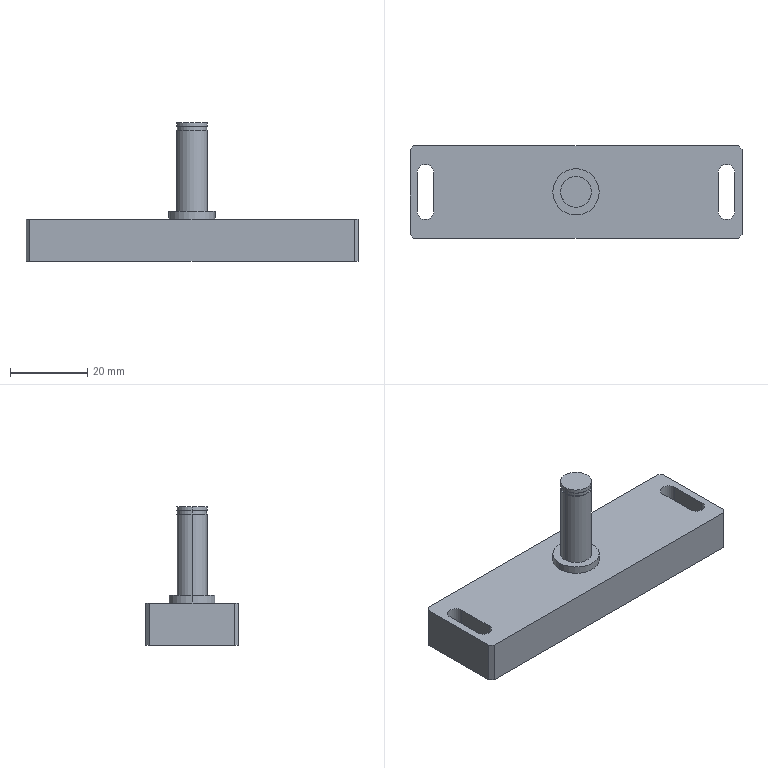Part | SolidWorks | features ICE 7, Chamfer 1, Extrusion 1, RevCut 1 | 1 solid | 30 faces | box 86 x 24 x 36 mm | volume 22794 mm3 | plane 18 | cylinder 12 | commonest cylinder face diameters 4.3 x4 8 x4 7.6 x2 12 x2
STEP:
#1=CARTESIAN_POINT('',(-4.,0.,28.5));
#2=VERTEX_POINT('',#1);
#3=CARTESIAN_POINT('',(4.,0.,28.5));
#4=VERTEX_POINT('',#3);
#5=CARTESIAN_POINT('',(0.,0.,28.5));
#6=DIRECTION('',(0.,0.,-1.));
#7=DIRECTION('',(-1.,0.,0.));
#8=AXIS2_PLACEMENT_3D('',#5,#6,#7);
#9=CIRCLE('',#8,4.);
#10=EDGE_CURVE('',#2,#4,#9,.T.);
#11=ORIENTED_EDGE('',*,*,#10,.T.);
#12=CARTESIAN_POINT('',(4.,0.,7.5));
#13=VERTEX_POINT('',#12);
#14=CARTESIAN_POINT('',(4.,0.,9.));
#15=DIRECTION('',(0.,0.,-1.));
#16=VECTOR('',#15,1000.);
#17=LINE('',#14,#16);
#18=EDGE_CURVE('',#4,#13,#17,.T.);
#19=ORIENTED_EDGE('',*,*,#18,.T.);
#20=CARTESIAN_POINT('',(-4.,0.,7.5));
#21=VERTEX_POINT('',#20);
#22=CARTESIAN_POINT('',(0.,0.,7.5));
#23=DIRECTION('',(0.,0.,1.));
#24=DIRECTION('',(1.,0.,0.));
#25=AXIS2_PLACEMENT_3D('',#22,#23,#24);
#26=CIRCLE('',#25,4.);
#27=EDGE_CURVE('',#13,#21,#26,.T.);
#28=ORIENTED_EDGE('',*,*,#27,.T.);
#29=CARTESIAN_POINT('',(-4.,0.,9.));
#30=DIRECTION('',(0.,0.,-1.));
#31=VECTOR('',#30,1000.);
#32=LINE('',#29,#31);
#33=EDGE_CURVE('',#2,#21,#32,.T.);
#34=ORIENTED_EDGE('',*,*,#33,.F.);
#35=EDGE_LOOP('',(#11,#19,#28,#34));
#36=FACE_OUTER_BOUND('',#35,.T.);
#37=CARTESIAN_POINT('',(0.,0.,9.));
#38=DIRECTION('',(0.,0.,-1.));
#39=DIRECTION('',(-1.,0.,0.));
#40=AXIS2_PLACEMENT_3D('',#37,#38,#39);
#41=CYLINDRICAL_SURFACE('',#40,4.);
#42=ADVANCED_FACE('',(#36),#41,.T.);
#43=CARTESIAN_POINT('',(-3.8,0.,29.5));
#44=VERTEX_POINT('',#43);
#45=CARTESIAN_POINT('',(3.8,0.,29.5));
#46=VERTEX_POINT('',#45);
#47=CARTESIAN_POINT('',(0.,0.,29.5));
#48=DIRECTION('',(0.,0.,-1.));
#49=DIRECTION('',(-1.,0.,0.));
#50=AXIS2_PLACEMENT_3D('',#47,#48,#49);
#51=CIRCLE('',#50,3.8);
#52=EDGE_CURVE('',#44,#46,#51,.T.);
#53=ORIENTED_EDGE('',*,*,#52,.T.);
#54=CARTESIAN_POINT('',(3.8,0.,28.5));
#55=VERTEX_POINT('',#54);
#56=CARTESIAN_POINT('',(3.8,0.,0.));
#57=DIRECTION('',(0.,0.,-1.));
#58=VECTOR('',#57,1000.);
#59=LINE('',#56,#58);
#60=EDGE_CURVE('',#46,#55,#59,.T.);
#61=ORIENTED_EDGE('',*,*,#60,.T.);
#62=CARTESIAN_POINT('',(-3.8,0.,28.5));
#63=VERTEX_POINT('',#62);
#64=CARTESIAN_POINT('',(0.,0.,28.5));
#65=DIRECTION('',(0.,0.,-1.));
#66=DIRECTION('',(-1.,0.,0.));
#67=AXIS2_PLACEMENT_3D('',#64,#65,#66);
#68=CIRCLE('',#67,3.8);
#69=EDGE_CURVE('',#63,#55,#68,.T.);
#70=ORIENTED_EDGE('',*,*,#69,.F.);
#71=CARTESIAN_POINT('',(-3.8,0.,0.));
#72=DIRECTION('',(0.,0.,-1.));
#73=VECTOR('',#72,1000.);
#74=LINE('',#71,#73);
#75=EDGE_CURVE('',#44,#63,#74,.T.);
#76=ORIENTED_EDGE('',*,*,#75,.F.);
#77=EDGE_LOOP('',(#53,#61,#70,#76));
#78=FACE_OUTER_BOUND('',#77,.T.);
#79=CARTESIAN_POINT('',(0.,0.,0.));
#80=DIRECTION('',(0.,0.,-1.));
#81=DIRECTION('',(-1.,0.,0.));
#82=AXIS2_PLACEMENT_3D('',#79,#80,#81);
#83=CYLINDRICAL_SURFACE('',#82,3.8);
#84=ADVANCED_FACE('',(#78),#83,.T.);
#85=CARTESIAN_POINT('',(4.,0.,30.5));
#86=VERTEX_POINT('',#85);
#87=CARTESIAN_POINT('',(-4.,0.,30.5));
#88=VERTEX_POINT('',#87);
#89=CARTESIAN_POINT('',(0.,0.,30.5));
#90=DIRECTION('',(0.,0.,1.));
#91=DIRECTION('',(1.,0.,0.));
#92=AXIS2_PLACEMENT_3D('',#89,#90,#91);
#93=CIRCLE('',#92,4.);
#94=EDGE_CURVE('',#86,#88,#93,.T.);
#95=ORIENTED_EDGE('',*,*,#94,.F.);
#96=CARTESIAN_POINT('',(4.,0.,29.5));
#97=VERTEX_POINT('',#96);
#98=CARTESIAN_POINT('',(4.,0.,9.));
#99=DIRECTION('',(0.,0.,-1.));
#100=VECTOR('',#99,1000.);
#101=LINE('',#98,#100);
#102=EDGE_CURVE('',#86,#97,#101,.T.);
#103=ORIENTED_EDGE('',*,*,#102,.T.);
#104=CARTESIAN_POINT('',(-4.,0.,29.5));
#105=VERTEX_POINT('',#104);
#106=CARTESIAN_POINT('',(0.,0.,29.5));
#107=DIRECTION('',(0.,0.,-1.));
#108=DIRECTION('',(-1.,0.,0.));
#109=AXIS2_PLACEMENT_3D('',#106,#107,#108);
#110=CIRCLE('',#109,4.);
#111=EDGE_CURVE('',#105,#97,#110,.T.);
#112=ORIENTED_EDGE('',*,*,#111,.F.);
#113=CARTESIAN_POINT('',(-4.,0.,9.));
#114=DIRECTION('',(0.,0.,-1.));
#115=VECTOR('',#114,1000.);
#116=LINE('',#113,#115);
#117=EDGE_CURVE('',#88,#105,#116,.T.);
#118=ORIENTED_EDGE('',*,*,#117,.F.);
#119=EDGE_LOOP('',(#95,#103,#112,#118));
#120=FACE_OUTER_BOUND('',#119,.T.);
#121=CARTESIAN_POINT('',(0.,0.,9.));
#122=DIRECTION('',(0.,0.,-1.));
#123=DIRECTION('',(-1.,0.,0.));
#124=AXIS2_PLACEMENT_3D('',#121,#122,#123);
#125=CYLINDRICAL_SURFACE('',#124,4.);
#126=ADVANCED_FACE('',(#120),#125,.T.);
#127=CARTESIAN_POINT('',(6.,0.,7.5));
#128=VERTEX_POINT('',#127);
#129=CARTESIAN_POINT('',(-6.,0.,7.5));
#130=VERTEX_POINT('',#129);
#131=CARTESIAN_POINT('',(0.,0.,7.5));
#132=DIRECTION('',(0.,0.,1.));
#133=DIRECTION('',(1.,0.,0.));
#134=AXIS2_PLACEMENT_3D('',#131,#132,#133);
#135=CIRCLE('',#134,6.);
#136=EDGE_CURVE('',#128,#130,#135,.T.);
#137=ORIENTED_EDGE('',*,*,#136,.F.);
#138=CARTESIAN_POINT('',(6.,0.,5.5));
#139=VERTEX_POINT('',#138);
#140=CARTESIAN_POINT('',(6.,0.,7.5));
#141=DIRECTION('',(0.,0.,-1.));
#142=VECTOR('',#141,1000.);
#143=LINE('',#140,#142);
#144=EDGE_CURVE('',#128,#139,#143,.T.);
#145=ORIENTED_EDGE('',*,*,#144,.T.);
#146=CARTESIAN_POINT('',(-6.,0.,5.5));
#147=VERTEX_POINT('',#146);
#148=CARTESIAN_POINT('',(0.,0.,5.5));
#149=DIRECTION('',(0.,0.,1.));
#150=DIRECTION('',(1.,0.,0.));
#151=AXIS2_PLACEMENT_3D('',#148,#149,#150);
#152=CIRCLE('',#151,6.);
#153=EDGE_CURVE('',#139,#147,#152,.T.);
#154=ORIENTED_EDGE('',*,*,#153,.T.);
#155=CARTESIAN_POINT('',(-6.,0.,7.5));
#156=DIRECTION('',(0.,0.,-1.));
#157=VECTOR('',#156,1000.);
#158=LINE('',#155,#157);
#159=EDGE_CURVE('',#130,#147,#158,.T.);
#160=ORIENTED_EDGE('',*,*,#159,.F.);
#161=EDGE_LOOP('',(#137,#145,#154,#160));
#162=FACE_OUTER_BOUND('',#161,.T.);
#163=CARTESIAN_POINT('',(0.,0.,7.5));
#164=DIRECTION('',(0.,0.,-1.));
#165=DIRECTION('',(-1.,0.,0.));
#166=AXIS2_PLACEMENT_3D('',#163,#164,#165);
#167=CYLINDRICAL_SURFACE('',#166,6.);
#168=ADVANCED_FACE('',(#162),#167,.T.);
#169=CARTESIAN_POINT('',(43.,-11.,5.5));
#170=VERTEX_POINT('',#169);
#171=CARTESIAN_POINT('',(43.,11.,5.5));
#172=VERTEX_POINT('',#171);
#173=CARTESIAN_POINT('',(43.,12.,5.5));
#174=DIRECTION('',(0.,1.,0.));
#175=VECTOR('',#174,1000.);
#176=LINE('',#173,#175);
#177=EDGE_CURVE('',#170,#172,#176,.T.);
#178=ORIENTED_EDGE('',*,*,#177,.T.);
#179=CARTESIAN_POINT('',(42.,12.,5.5));
#180=VERTEX_POINT('',#179);
#181=CARTESIAN_POINT('',(27.,27.,5.5));
#182=DIRECTION('',(-0.7071,0.7071,0.));
#183=VECTOR('',#182,1000.);
#184=LINE('',#181,#183);
#185=EDGE_CURVE('',#172,#180,#184,.T.);
#186=ORIENTED_EDGE('',*,*,#185,.T.);
#187=CARTESIAN_POINT('',(-42.,12.,5.5));
#188=VERTEX_POINT('',#187);
#189=CARTESIAN_POINT('',(-43.,12.,5.5));
#190=DIRECTION('',(-1.,0.,0.));
#191=VECTOR('',#190,1000.);
#192=LINE('',#189,#191);
#193=EDGE_CURVE('',#180,#188,#192,.T.);
#194=ORIENTED_EDGE('',*,*,#193,.T.);
#195=CARTESIAN_POINT('',(-43.,11.,5.5));
#196=VERTEX_POINT('',#195);
#197=CARTESIAN_POINT('',(-27.,27.,5.5));
#198=DIRECTION('',(-0.7071,-0.7071,0.));
#199=VECTOR('',#198,1000.);
#200=LINE('',#197,#199);
#201=EDGE_CURVE('',#188,#196,#200,.T.);
#202=ORIENTED_EDGE('',*,*,#201,.T.);
#203=CARTESIAN_POINT('',(-43.,-11.,5.5));
#204=VERTEX_POINT('',#203);
#205=CARTESIAN_POINT('',(-43.,12.,5.5));
#206=DIRECTION('',(0.,-1.,0.));
#207=VECTOR('',#206,1000.);
#208=LINE('',#205,#207);
#209=EDGE_CURVE('',#196,#204,#208,.T.);
#210=ORIENTED_EDGE('',*,*,#209,.T.);
#211=CARTESIAN_POINT('',(-42.,-12.,5.5));
#212=VERTEX_POINT('',#211);
#213=CARTESIAN_POINT('',(-27.,-27.,5.5));
#214=DIRECTION('',(0.7071,-0.7071,0.));
#215=VECTOR('',#214,1000.);
#216=LINE('',#213,#215);
#217=EDGE_CURVE('',#204,#212,#216,.T.);
#218=ORIENTED_EDGE('',*,*,#217,.T.);
#219=CARTESIAN_POINT('',(42.,-12.,5.5));
#220=VERTEX_POINT('',#219);
#221=CARTESIAN_POINT('',(-43.,-12.,5.5));
#222=DIRECTION('',(1.,0.,0.));
#223=VECTOR('',#222,1000.);
#224=LINE('',#221,#223);
#225=EDGE_CURVE('',#212,#220,#224,.T.);
#226=ORIENTED_EDGE('',*,*,#225,.T.);
#227=CARTESIAN_POINT('',(27.,-27.,5.5));
#228=DIRECTION('',(0.7071,0.7071,0.));
#229=VECTOR('',#228,1000.);
#230=LINE('',#227,#229);
#231=EDGE_CURVE('',#220,#170,#230,.T.);
#232=ORIENTED_EDGE('',*,*,#231,.T.);
#233=EDGE_LOOP('',(#178,#186,#194,#202,#210,#218,#226,#232));
#234=FACE_OUTER_BOUND('',#233,.T.);
#235=CARTESIAN_POINT('',(41.15,5.,5.5));
#236=VERTEX_POINT('',#235);
#237=CARTESIAN_POINT('',(36.85,5.,5.5));
#238=VERTEX_POINT('',#237);
#239=CARTESIAN_POINT('',(39.,5.,5.5));
#240=DIRECTION('',(0.,0.,1.));
#241=DIRECTION('',(1.,0.,0.));
#242=AXIS2_PLACEMENT_3D('',#239,#240,#241);
#243=CIRCLE('',#242,2.15);
#244=EDGE_CURVE('',#236,#238,#243,.T.);
#245=ORIENTED_EDGE('',*,*,#244,.F.);
#246=CARTESIAN_POINT('',(41.15,-5.,5.5));
#247=VERTEX_POINT('',#246);
#248=CARTESIAN_POINT('',(41.15,0.,5.5));
#249=DIRECTION('',(0.,1.,0.));
#250=VECTOR('',#249,1000.);
#251=LINE('',#248,#250);
#252=EDGE_CURVE('',#247,#236,#251,.T.);
#253=ORIENTED_EDGE('',*,*,#252,.F.);
#254=CARTESIAN_POINT('',(36.85,-5.,5.5));
#255=VERTEX_POINT('',#254);
#256=CARTESIAN_POINT('',(39.,-5.,5.5));
#257=DIRECTION('',(0.,0.,1.));
#258=DIRECTION('',(1.,0.,0.));
#259=AXIS2_PLACEMENT_3D('',#256,#257,#258);
#260=CIRCLE('',#259,2.15);
#261=EDGE_CURVE('',#255,#247,#260,.T.);
#262=ORIENTED_EDGE('',*,*,#261,.F.);
#263=CARTESIAN_POINT('',(36.85,0.,5.5));
#264=DIRECTION('',(0.,-1.,0.));
#265=VECTOR('',#264,1000.);
#266=LINE('',#263,#265);
#267=EDGE_CURVE('',#238,#255,#266,.T.);
#268=ORIENTED_EDGE('',*,*,#267,.F.);
#269=EDGE_LOOP('',(#245,#253,#262,#268));
#270=FACE_BOUND('',#269,.T.);
#271=CARTESIAN_POINT('',(-36.85,5.,5.5));
#272=VERTEX_POINT('',#271);
#273=CARTESIAN_POINT('',(-41.15,5.,5.5));
#274=VERTEX_POINT('',#273);
#275=CARTESIAN_POINT('',(-39.,5.,5.5));
#276=DIRECTION('',(0.,0.,1.));
#277=DIRECTION('',(1.,0.,0.));
#278=AXIS2_PLACEMENT_3D('',#275,#276,#277);
#279=CIRCLE('',#278,2.15);
#280=EDGE_CURVE('',#272,#274,#279,.T.);
#281=ORIENTED_EDGE('',*,*,#280,.F.);
#282=CARTESIAN_POINT('',(-36.85,-5.,5.5));
#283=VERTEX_POINT('',#282);
#284=CARTESIAN_POINT('',(-36.85,0.,5.5));
#285=DIRECTION('',(0.,1.,0.));
#286=VECTOR('',#285,1000.);
#287=LINE('',#284,#286);
#288=EDGE_CURVE('',#283,#272,#287,.T.);
#289=ORIENTED_EDGE('',*,*,#288,.F.);
#290=CARTESIAN_POINT('',(-41.15,-5.,5.5));
#291=VERTEX_POINT('',#290);
#292=CARTESIAN_POINT('',(-39.,-5.,5.5));
#293=DIRECTION('',(0.,0.,1.));
#294=DIRECTION('',(1.,0.,0.));
#295=AXIS2_PLACEMENT_3D('',#292,#293,#294);
#296=CIRCLE('',#295,2.15);
#297=EDGE_CURVE('',#291,#283,#296,.T.);
#298=ORIENTED_EDGE('',*,*,#297,.F.);
#299=CARTESIAN_POINT('',(-41.15,0.,5.5));
#300=DIRECTION('',(0.,-1.,0.));
#301=VECTOR('',#300,1000.);
#302=LINE('',#299,#301);
#303=EDGE_CURVE('',#274,#291,#302,.T.);
#304=ORIENTED_EDGE('',*,*,#303,.F.);
#305=EDGE_LOOP('',(#281,#289,#298,#304));
#306=FACE_BOUND('',#305,.T.);
#307=CARTESIAN_POINT('',(0.,0.,5.5));
#308=DIRECTION('',(0.,0.,1.));
#309=DIRECTION('',(1.,0.,0.));
#310=AXIS2_PLACEMENT_3D('',#307,#308,#309);
#311=CIRCLE('',#310,6.);
#312=EDGE_CURVE('',#147,#139,#311,.T.);
#313=ORIENTED_EDGE('',*,*,#312,.F.);
#314=ORIENTED_EDGE('',*,*,#153,.F.);
#315=EDGE_LOOP('',(#313,#314));
#316=FACE_BOUND('',#315,.T.);
#317=CARTESIAN_POINT('',(0.,0.,5.5));
#318=DIRECTION('',(0.,0.,1.));
#319=DIRECTION('',(1.,0.,0.));
#320=AXIS2_PLACEMENT_3D('',#317,#318,#319);
#321=PLANE('',#320);
#322=ADVANCED_FACE('',(#234,#270,#306,#316),#321,.T.);
#323=CARTESIAN_POINT('',(43.,-11.,-5.5));
#324=VERTEX_POINT('',#323);
#325=CARTESIAN_POINT('',(43.,11.,-5.5));
#326=VERTEX_POINT('',#325);
#327=CARTESIAN_POINT('',(43.,12.,-5.5));
#328=DIRECTION('',(0.,1.,0.));
#329=VECTOR('',#328,1000.);
#330=LINE('',#327,#329);
#331=EDGE_CURVE('',#324,#326,#330,.T.);
#332=ORIENTED_EDGE('',*,*,#331,.T.);
#333=CARTESIAN_POINT('',(43.,11.,5.5));
#334=DIRECTION('',(0.,0.,1.));
#335=VECTOR('',#334,1000.);
#336=LINE('',#333,#335);
#337=EDGE_CURVE('',#326,#172,#336,.T.);
#338=ORIENTED_EDGE('',*,*,#337,.T.);
#339=ORIENTED_EDGE('',*,*,#177,.F.);
#340=CARTESIAN_POINT('',(43.,-11.,5.5));
#341=DIRECTION('',(0.,0.,-1.));
#342=VECTOR('',#341,1000.);
#343=LINE('',#340,#342);
#344=EDGE_CURVE('',#170,#324,#343,.T.);
#345=ORIENTED_EDGE('',*,*,#344,.T.);
#346=EDGE_LOOP('',(#332,#338,#339,#345));
#347=FACE_OUTER_BOUND('',#346,.T.);
#348=CARTESIAN_POINT('',(43.,12.,5.5));
#349=DIRECTION('',(-1.,0.,0.));
#350=DIRECTION('',(0.,0.,1.));
#351=AXIS2_PLACEMENT_3D('',#348,#349,#350);
#352=PLANE('',#351);
#353=ADVANCED_FACE('',(#347),#352,.F.);
#354=ORIENTED_EDGE('',*,*,#193,.F.);
#355=CARTESIAN_POINT('',(42.,12.,-5.5));
#356=VERTEX_POINT('',#355);
#357=CARTESIAN_POINT('',(42.,12.,5.5));
#358=DIRECTION('',(0.,0.,-1.));
#359=VECTOR('',#358,1000.);
#360=LINE('',#357,#359);
#361=EDGE_CURVE('',#180,#356,#360,.T.);
#362=ORIENTED_EDGE('',*,*,#361,.T.);
#363=CARTESIAN_POINT('',(-42.,12.,-5.5));
#364=VERTEX_POINT('',#363);
#365=CARTESIAN_POINT('',(-43.,12.,-5.5));
#366=DIRECTION('',(-1.,0.,0.));
#367=VECTOR('',#366,1000.);
#368=LINE('',#365,#367);
#369=EDGE_CURVE('',#356,#364,#368,.T.);
#370=ORIENTED_EDGE('',*,*,#369,.T.);
#371=CARTESIAN_POINT('',(-42.,12.,5.5));
#372=DIRECTION('',(0.,0.,1.));
#373=VECTOR('',#372,1000.);
#374=LINE('',#371,#373);
#375=EDGE_CURVE('',#364,#188,#374,.T.);
#376=ORIENTED_EDGE('',*,*,#375,.T.);
#377=EDGE_LOOP('',(#354,#362,#370,#376));
#378=FACE_OUTER_BOUND('',#377,.T.);
#379=CARTESIAN_POINT('',(-43.,12.,5.5));
#380=DIRECTION('',(0.,-1.,0.));
#381=DIRECTION('',(0.,0.,-1.));
#382=AXIS2_PLACEMENT_3D('',#379,#380,#381);
#383=PLANE('',#382);
#384=ADVANCED_FACE('',(#378),#383,.F.);
#385=ORIENTED_EDGE('',*,*,#209,.F.);
#386=CARTESIAN_POINT('',(-43.,11.,-5.5));
#387=VERTEX_POINT('',#386);
#388=CARTESIAN_POINT('',(-43.,11.,5.5));
#389=DIRECTION('',(0.,0.,-1.));
#390=VECTOR('',#389,1000.);
#391=LINE('',#388,#390);
#392=EDGE_CURVE('',#196,#387,#391,.T.);
#393=ORIENTED_EDGE('',*,*,#392,.T.);
#394=CARTESIAN_POINT('',(-43.,-11.,-5.5));
#395=VERTEX_POINT('',#394);
#396=CARTESIAN_POINT('',(-43.,12.,-5.5));
#397=DIRECTION('',(0.,-1.,0.));
#398=VECTOR('',#397,1000.);
#399=LINE('',#396,#398);
#400=EDGE_CURVE('',#387,#395,#399,.T.);
#401=ORIENTED_EDGE('',*,*,#400,.T.);
#402=CARTESIAN_POINT('',(-43.,-11.,5.5));
#403=DIRECTION('',(0.,0.,1.));
#404=VECTOR('',#403,1000.);
#405=LINE('',#402,#404);
#406=EDGE_CURVE('',#395,#204,#405,.T.);
#407=ORIENTED_EDGE('',*,*,#406,.T.);
#408=EDGE_LOOP('',(#385,#393,#401,#407));
#409=FACE_OUTER_BOUND('',#408,.T.);
#410=CARTESIAN_POINT('',(-43.,12.,5.5));
#411=DIRECTION('',(1.,0.,0.));
#412=DIRECTION('',(0.,0.,-1.));
#413=AXIS2_PLACEMENT_3D('',#410,#411,#412);
#414=PLANE('',#413);
#415=ADVANCED_FACE('',(#409),#414,.F.);
#416=ORIENTED_EDGE('',*,*,#225,.F.);
#417=CARTESIAN_POINT('',(-42.,-12.,-5.5));
#418=VERTEX_POINT('',#417);
#419=CARTESIAN_POINT('',(-42.,-12.,5.5));
#420=DIRECTION('',(0.,0.,-1.));
#421=VECTOR('',#420,1000.);
#422=LINE('',#419,#421);
#423=EDGE_CURVE('',#212,#418,#422,.T.);
#424=ORIENTED_EDGE('',*,*,#423,.T.);
#425=CARTESIAN_POINT('',(42.,-12.,-5.5));
#426=VERTEX_POINT('',#425);
#427=CARTESIAN_POINT('',(-43.,-12.,-5.5));
#428=DIRECTION('',(1.,0.,0.));
#429=VECTOR('',#428,1000.);
#430=LINE('',#427,#429);
#431=EDGE_CURVE('',#418,#426,#430,.T.);
#432=ORIENTED_EDGE('',*,*,#431,.T.);
#433=CARTESIAN_POINT('',(42.,-12.,5.5));
#434=DIRECTION('',(0.,0.,1.));
#435=VECTOR('',#434,1000.);
#436=LINE('',#433,#435);
#437=EDGE_CURVE('',#426,#220,#436,.T.);
#438=ORIENTED_EDGE('',*,*,#437,.T.);
#439=EDGE_LOOP('',(#416,#424,#432,#438));
#440=FACE_OUTER_BOUND('',#439,.T.);
#441=CARTESIAN_POINT('',(-43.,-12.,5.5));
#442=DIRECTION('',(0.,1.,0.));
#443=DIRECTION('',(0.,0.,1.));
#444=AXIS2_PLACEMENT_3D('',#441,#442,#443);
#445=PLANE('',#444);
#446=ADVANCED_FACE('',(#440),#445,.F.);
#447=CARTESIAN_POINT('',(-36.85,5.,-5.5));
#448=VERTEX_POINT('',#447);
#449=CARTESIAN_POINT('',(-36.85,-5.,-5.5));
#450=VERTEX_POINT('',#449);
#451=CARTESIAN_POINT('',(-36.85,5.,-5.5));
#452=DIRECTION('',(0.,-1.,0.));
#453=VECTOR('',#452,1000.);
#454=LINE('',#451,#453);
#455=EDGE_CURVE('',#448,#450,#454,.T.);
#456=ORIENTED_EDGE('',*,*,#455,.F.);
#457=CARTESIAN_POINT('',(-41.15,5.,-5.5));
#458=VERTEX_POINT('',#457);
#459=CARTESIAN_POINT('',(-39.,5.,-5.5));
#460=DIRECTION('',(0.,0.,-1.));
#461=DIRECTION('',(1.,0.,0.));
#462=AXIS2_PLACEMENT_3D('',#459,#460,#461);
#463=CIRCLE('',#462,2.15);
#464=EDGE_CURVE('',#458,#448,#463,.T.);
#465=ORIENTED_EDGE('',*,*,#464,.F.);
#466=CARTESIAN_POINT('',(-41.15,-5.,-5.5));
#467=VERTEX_POINT('',#466);
#468=CARTESIAN_POINT('',(-41.15,5.,-5.5));
#469=DIRECTION('',(0.,1.,0.));
#470=VECTOR('',#469,1000.);
#471=LINE('',#468,#470);
#472=EDGE_CURVE('',#467,#458,#471,.T.);
#473=ORIENTED_EDGE('',*,*,#472,.F.);
#474=CARTESIAN_POINT('',(-39.,-5.,-5.5));
#475=DIRECTION('',(0.,0.,-1.));
#476=DIRECTION('',(1.,0.,0.));
#477=AXIS2_PLACEMENT_3D('',#474,#475,#476);
#478=CIRCLE('',#477,2.15);
#479=EDGE_CURVE('',#450,#467,#478,.T.);
#480=ORIENTED_EDGE('',*,*,#479,.F.);
#481=EDGE_LOOP('',(#456,#465,#473,#480));
#482=FACE_BOUND('',#481,.T.);
#483=CARTESIAN_POINT('',(41.15,5.,-5.5));
#484=VERTEX_POINT('',#483);
#485=CARTESIAN_POINT('',(41.15,-5.,-5.5));
#486=VERTEX_POINT('',#485);
#487=CARTESIAN_POINT('',(41.15,5.,-5.5));
#488=DIRECTION('',(0.,-1.,0.));
#489=VECTOR('',#488,1000.);
#490=LINE('',#487,#489);
#491=EDGE_CURVE('',#484,#486,#490,.T.);
#492=ORIENTED_EDGE('',*,*,#491,.F.);
#493=CARTESIAN_POINT('',(36.85,5.,-5.5));
#494=VERTEX_POINT('',#493);
#495=CARTESIAN_POINT('',(39.,5.,-5.5));
#496=DIRECTION('',(0.,0.,-1.));
#497=DIRECTION('',(-1.,0.,0.));
#498=AXIS2_PLACEMENT_3D('',#495,#496,#497);
#499=CIRCLE('',#498,2.15);
#500=EDGE_CURVE('',#494,#484,#499,.T.);
#501=ORIENTED_EDGE('',*,*,#500,.F.);
#502=CARTESIAN_POINT('',(36.85,-5.,-5.5));
#503=VERTEX_POINT('',#502);
#504=CARTESIAN_POINT('',(36.85,5.,-5.5));
#505=DIRECTION('',(0.,1.,0.));
#506=VECTOR('',#505,1000.);
#507=LINE('',#504,#506);
#508=EDGE_CURVE('',#503,#494,#507,.T.);
#509=ORIENTED_EDGE('',*,*,#508,.F.);
#510=CARTESIAN_POINT('',(39.,-5.,-5.5));
#511=DIRECTION('',(0.,0.,-1.));
#512=DIRECTION('',(-1.,0.,0.));
#513=AXIS2_PLACEMENT_3D('',#510,#511,#512);
#514=CIRCLE('',#513,2.15);
#515=EDGE_CURVE('',#486,#503,#514,.T.);
#516=ORIENTED_EDGE('',*,*,#515,.F.);
#517=EDGE_LOOP('',(#492,#501,#509,#516));
#518=FACE_BOUND('',#517,.T.);
#519=ORIENTED_EDGE('',*,*,#369,.F.);
#520=CARTESIAN_POINT('',(42.,12.,-5.5));
#521=DIRECTION('',(0.7071,-0.7071,0.));
#522=VECTOR('',#521,1000.);
#523=LINE('',#520,#522);
#524=EDGE_CURVE('',#356,#326,#523,.T.);
#525=ORIENTED_EDGE('',*,*,#524,.T.);
#526=ORIENTED_EDGE('',*,*,#331,.F.);
#527=CARTESIAN_POINT('',(43.,-11.,-5.5));
#528=DIRECTION('',(-0.7071,-0.7071,0.));
#529=VECTOR('',#528,1000.);
#530=LINE('',#527,#529);
#531=EDGE_CURVE('',#324,#426,#530,.T.);
#532=ORIENTED_EDGE('',*,*,#531,.T.);
#533=ORIENTED_EDGE('',*,*,#431,.F.);
#534=CARTESIAN_POINT('',(-42.,-12.,-5.5));
#535=DIRECTION('',(-0.7071,0.7071,0.));
#536=VECTOR('',#535,1000.);
#537=LINE('',#534,#536);
#538=EDGE_CURVE('',#418,#395,#537,.T.);
#539=ORIENTED_EDGE('',*,*,#538,.T.);
#540=ORIENTED_EDGE('',*,*,#400,.F.);
#541=CARTESIAN_POINT('',(-43.,11.,-5.5));
#542=DIRECTION('',(0.7071,0.7071,0.));
#543=VECTOR('',#542,1000.);
#544=LINE('',#541,#543);
#545=EDGE_CURVE('',#387,#364,#544,.T.);
#546=ORIENTED_EDGE('',*,*,#545,.T.);
#547=EDGE_LOOP('',(#519,#525,#526,#532,#533,#539,#540,#546));
#548=FACE_OUTER_BOUND('',#547,.T.);
#549=CARTESIAN_POINT('',(0.,0.,-5.5));
#550=DIRECTION('',(0.,0.,1.));
#551=DIRECTION('',(1.,0.,0.));
#552=AXIS2_PLACEMENT_3D('',#549,#550,#551);
#553=PLANE('',#552);
#554=ADVANCED_FACE('',(#482,#518,#548),#553,.F.);
#555=ORIENTED_EDGE('',*,*,#244,.T.);
#556=CARTESIAN_POINT('',(36.85,5.,30.5));
#557=DIRECTION('',(0.,0.,-1.));
#558=VECTOR('',#557,1000.);
#559=LINE('',#556,#558);
#560=EDGE_CURVE('',#238,#494,#559,.T.);
#561=ORIENTED_EDGE('',*,*,#560,.T.);
#562=ORIENTED_EDGE('',*,*,#500,.T.);
#563=CARTESIAN_POINT('',(41.15,5.,30.5));
#564=DIRECTION('',(0.,0.,-1.));
#565=VECTOR('',#564,1000.);
#566=LINE('',#563,#565);
#567=EDGE_CURVE('',#236,#484,#566,.T.);
#568=ORIENTED_EDGE('',*,*,#567,.F.);
#569=EDGE_LOOP('',(#555,#561,#562,#568));
#570=FACE_OUTER_BOUND('',#569,.T.);
#571=CARTESIAN_POINT('',(39.,5.,30.5));
#572=DIRECTION('',(0.,0.,-1.));
#573=DIRECTION('',(-1.,0.,0.));
#574=AXIS2_PLACEMENT_3D('',#571,#572,#573);
#575=CYLINDRICAL_SURFACE('',#574,2.15);
#576=ADVANCED_FACE('',(#570),#575,.F.);
#577=ORIENTED_EDGE('',*,*,#267,.T.);
#578=CARTESIAN_POINT('',(36.85,-5.,30.5));
#579=DIRECTION('',(0.,0.,-1.));
#580=VECTOR('',#579,1000.);
#581=LINE('',#578,#580);
#582=EDGE_CURVE('',#255,#503,#581,.T.);
#583=ORIENTED_EDGE('',*,*,#582,.T.);
#584=ORIENTED_EDGE('',*,*,#508,.T.);
#585=ORIENTED_EDGE('',*,*,#560,.F.);
#586=EDGE_LOOP('',(#577,#583,#584,#585));
#587=FACE_OUTER_BOUND('',#586,.T.);
#588=CARTESIAN_POINT('',(36.85,5.,30.5));
#589=DIRECTION('',(-1.,0.,0.));
#590=DIRECTION('',(0.,0.,1.));
#591=AXIS2_PLACEMENT_3D('',#588,#589,#590);
#592=PLANE('',#591);
#593=ADVANCED_FACE('',(#587),#592,.F.);
#594=ORIENTED_EDGE('',*,*,#261,.T.);
#595=CARTESIAN_POINT('',(41.15,-5.,30.5));
#596=DIRECTION('',(0.,0.,-1.));
#597=VECTOR('',#596,1000.);
#598=LINE('',#595,#597);
#599=EDGE_CURVE('',#247,#486,#598,.T.);
#600=ORIENTED_EDGE('',*,*,#599,.T.);
#601=ORIENTED_EDGE('',*,*,#515,.T.);
#602=ORIENTED_EDGE('',*,*,#582,.F.);
#603=EDGE_LOOP('',(#594,#600,#601,#602));
#604=FACE_OUTER_BOUND('',#603,.T.);
#605=CARTESIAN_POINT('',(39.,-5.,30.5));
#606=DIRECTION('',(0.,0.,-1.));
#607=DIRECTION('',(-1.,0.,0.));
#608=AXIS2_PLACEMENT_3D('',#605,#606,#607);
#609=CYLINDRICAL_SURFACE('',#608,2.15);
#610=ADVANCED_FACE('',(#604),#609,.F.);
#611=ORIENTED_EDGE('',*,*,#252,.T.);
#612=ORIENTED_EDGE('',*,*,#567,.T.);
#613=ORIENTED_EDGE('',*,*,#491,.T.);
#614=ORIENTED_EDGE('',*,*,#599,.F.);
#615=EDGE_LOOP('',(#611,#612,#613,#614));
#616=FACE_OUTER_BOUND('',#615,.T.);
#617=CARTESIAN_POINT('',(41.15,5.,30.5));
#618=DIRECTION('',(1.,0.,0.));
#619=DIRECTION('',(0.,0.,-1.));
#620=AXIS2_PLACEMENT_3D('',#617,#618,#619);
#621=PLANE('',#620);
#622=ADVANCED_FACE('',(#616),#621,.F.);
#623=ORIENTED_EDGE('',*,*,#280,.T.);
#624=CARTESIAN_POINT('',(-41.15,5.,30.5));
#625=DIRECTION('',(0.,0.,-1.));
#626=VECTOR('',#625,1000.);
#627=LINE('',#624,#626);
#628=EDGE_CURVE('',#274,#458,#627,.T.);
#629=ORIENTED_EDGE('',*,*,#628,.T.);
#630=ORIENTED_EDGE('',*,*,#464,.T.);
#631=CARTESIAN_POINT('',(-36.85,5.,30.5));
#632=DIRECTION('',(0.,0.,-1.));
#633=VECTOR('',#632,1000.);
#634=LINE('',#631,#633);
#635=EDGE_CURVE('',#272,#448,#634,.T.);
#636=ORIENTED_EDGE('',*,*,#635,.F.);
#637=EDGE_LOOP('',(#623,#629,#630,#636));
#638=FACE_OUTER_BOUND('',#637,.T.);
#639=CARTESIAN_POINT('',(-39.,5.,30.5));
#640=DIRECTION('',(0.,0.,-1.));
#641=DIRECTION('',(-1.,0.,0.));
#642=AXIS2_PLACEMENT_3D('',#639,#640,#641);
#643=CYLINDRICAL_SURFACE('',#642,2.15);
#644=ADVANCED_FACE('',(#638),#643,.F.);
#645=ORIENTED_EDGE('',*,*,#303,.T.);
#646=CARTESIAN_POINT('',(-41.15,-5.,30.5));
#647=DIRECTION('',(0.,0.,-1.));
#648=VECTOR('',#647,1000.);
#649=LINE('',#646,#648);
#650=EDGE_CURVE('',#291,#467,#649,.T.);
#651=ORIENTED_EDGE('',*,*,#650,.T.);
#652=ORIENTED_EDGE('',*,*,#472,.T.);
#653=ORIENTED_EDGE('',*,*,#628,.F.);
#654=EDGE_LOOP('',(#645,#651,#652,#653));
#655=FACE_OUTER_BOUND('',#654,.T.);
#656=CARTESIAN_POINT('',(-41.15,5.,30.5));
#657=DIRECTION('',(-1.,0.,0.));
#658=DIRECTION('',(0.,0.,1.));
#659=AXIS2_PLACEMENT_3D('',#656,#657,#658);
#660=PLANE('',#659);
#661=ADVANCED_FACE('',(#655),#660,.F.);
#662=ORIENTED_EDGE('',*,*,#297,.T.);
#663=CARTESIAN_POINT('',(-36.85,-5.,30.5));
#664=DIRECTION('',(0.,0.,-1.));
#665=VECTOR('',#664,1000.);
#666=LINE('',#663,#665);
#667=EDGE_CURVE('',#283,#450,#666,.T.);
#668=ORIENTED_EDGE('',*,*,#667,.T.);
#669=ORIENTED_EDGE('',*,*,#479,.T.);
#670=ORIENTED_EDGE('',*,*,#650,.F.);
#671=EDGE_LOOP('',(#662,#668,#669,#670));
#672=FACE_OUTER_BOUND('',#671,.T.);
#673=CARTESIAN_POINT('',(-39.,-5.,30.5));
#674=DIRECTION('',(0.,0.,-1.));
#675=DIRECTION('',(-1.,0.,0.));
#676=AXIS2_PLACEMENT_3D('',#673,#674,#675);
#677=CYLINDRICAL_SURFACE('',#676,2.15);
#678=ADVANCED_FACE('',(#672),#677,.F.);
#679=ORIENTED_EDGE('',*,*,#288,.T.);
#680=ORIENTED_EDGE('',*,*,#635,.T.);
#681=ORIENTED_EDGE('',*,*,#455,.T.);
#682=ORIENTED_EDGE('',*,*,#667,.F.);
#683=EDGE_LOOP('',(#679,#680,#681,#682));
#684=FACE_OUTER_BOUND('',#683,.T.);
#685=CARTESIAN_POINT('',(-36.85,5.,30.5));
#686=DIRECTION('',(1.,0.,0.));
#687=DIRECTION('',(0.,0.,-1.));
#688=AXIS2_PLACEMENT_3D('',#685,#686,#687);
#689=PLANE('',#688);
#690=ADVANCED_FACE('',(#684),#689,.F.);
#691=CARTESIAN_POINT('',(0.,0.,7.5));
#692=DIRECTION('',(0.,0.,1.));
#693=DIRECTION('',(1.,0.,0.));
#694=AXIS2_PLACEMENT_3D('',#691,#692,#693);
#695=CIRCLE('',#694,6.);
#696=EDGE_CURVE('',#130,#128,#695,.T.);
#697=ORIENTED_EDGE('',*,*,#696,.T.);
#698=ORIENTED_EDGE('',*,*,#136,.T.);
#699=EDGE_LOOP('',(#697,#698));
#700=FACE_OUTER_BOUND('',#699,.T.);
#701=CARTESIAN_POINT('',(0.,0.,7.5));
#702=DIRECTION('',(0.,0.,1.));
#703=DIRECTION('',(1.,0.,0.));
#704=AXIS2_PLACEMENT_3D('',#701,#702,#703);
#705=CIRCLE('',#704,4.);
#706=EDGE_CURVE('',#21,#13,#705,.T.);
#707=ORIENTED_EDGE('',*,*,#706,.F.);
#708=ORIENTED_EDGE('',*,*,#27,.F.);
#709=EDGE_LOOP('',(#707,#708));
#710=FACE_BOUND('',#709,.T.);
#711=CARTESIAN_POINT('',(0.,0.,7.5));
#712=DIRECTION('',(0.,0.,1.));
#713=DIRECTION('',(1.,0.,0.));
#714=AXIS2_PLACEMENT_3D('',#711,#712,#713);
#715=PLANE('',#714);
#716=ADVANCED_FACE('',(#700,#710),#715,.T.);
#717=ORIENTED_EDGE('',*,*,#144,.F.);
#718=ORIENTED_EDGE('',*,*,#696,.F.);
#719=ORIENTED_EDGE('',*,*,#159,.T.);
#720=ORIENTED_EDGE('',*,*,#312,.T.);
#721=EDGE_LOOP('',(#717,#718,#719,#720));
#722=FACE_OUTER_BOUND('',#721,.T.);
#723=CARTESIAN_POINT('',(0.,0.,7.5));
#724=DIRECTION('',(0.,0.,-1.));
#725=DIRECTION('',(-1.,0.,0.));
#726=AXIS2_PLACEMENT_3D('',#723,#724,#725);
#727=CYLINDRICAL_SURFACE('',#726,6.);
#728=ADVANCED_FACE('',(#722),#727,.T.);
#729=CARTESIAN_POINT('',(0.,0.,30.5));
#730=DIRECTION('',(0.,0.,1.));
#731=DIRECTION('',(1.,0.,0.));
#732=AXIS2_PLACEMENT_3D('',#729,#730,#731);
#733=CIRCLE('',#732,4.);
#734=EDGE_CURVE('',#88,#86,#733,.T.);
#735=ORIENTED_EDGE('',*,*,#734,.T.);
#736=ORIENTED_EDGE('',*,*,#94,.T.);
#737=EDGE_LOOP('',(#735,#736));
#738=FACE_OUTER_BOUND('',#737,.T.);
#739=CARTESIAN_POINT('',(0.,0.,30.5));
#740=DIRECTION('',(0.,0.,1.));
#741=DIRECTION('',(1.,0.,0.));
#742=AXIS2_PLACEMENT_3D('',#739,#740,#741);
#743=PLANE('',#742);
#744=ADVANCED_FACE('',(#738),#743,.T.);
#745=ORIENTED_EDGE('',*,*,#102,.F.);
#746=ORIENTED_EDGE('',*,*,#734,.F.);
#747=ORIENTED_EDGE('',*,*,#117,.T.);
#748=CARTESIAN_POINT('',(0.,0.,29.5));
#749=DIRECTION('',(0.,0.,-1.));
#750=DIRECTION('',(-1.,0.,0.));
#751=AXIS2_PLACEMENT_3D('',#748,#749,#750);
#752=CIRCLE('',#751,4.);
#753=EDGE_CURVE('',#97,#105,#752,.T.);
#754=ORIENTED_EDGE('',*,*,#753,.F.);
#755=EDGE_LOOP('',(#745,#746,#747,#754));
#756=FACE_OUTER_BOUND('',#755,.T.);
#757=CARTESIAN_POINT('',(0.,0.,9.));
#758=DIRECTION('',(0.,0.,-1.));
#759=DIRECTION('',(-1.,0.,0.));
#760=AXIS2_PLACEMENT_3D('',#757,#758,#759);
#761=CYLINDRICAL_SURFACE('',#760,4.);
#762=ADVANCED_FACE('',(#756),#761,.T.);
#763=ORIENTED_EDGE('',*,*,#52,.F.);
#764=CARTESIAN_POINT('',(0.,0.,29.5));
#765=DIRECTION('',(0.,0.,-1.));
#766=DIRECTION('',(-1.,0.,0.));
#767=AXIS2_PLACEMENT_3D('',#764,#765,#766);
#768=CIRCLE('',#767,3.8);
#769=EDGE_CURVE('',#46,#44,#768,.T.);
#770=ORIENTED_EDGE('',*,*,#769,.F.);
#771=EDGE_LOOP('',(#763,#770));
#772=FACE_BOUND('',#771,.T.);
#773=ORIENTED_EDGE('',*,*,#111,.T.);
#774=ORIENTED_EDGE('',*,*,#753,.T.);
#775=EDGE_LOOP('',(#773,#774));
#776=FACE_OUTER_BOUND('',#775,.T.);
#777=CARTESIAN_POINT('',(-4.,0.,29.5));
#778=DIRECTION('',(0.,0.,1.));
#779=DIRECTION('',(1.,0.,0.));
#780=AXIS2_PLACEMENT_3D('',#777,#778,#779);
#781=PLANE('',#780);
#782=ADVANCED_FACE('',(#772,#776),#781,.F.);
#783=ORIENTED_EDGE('',*,*,#60,.F.);
#784=ORIENTED_EDGE('',*,*,#769,.T.);
#785=ORIENTED_EDGE('',*,*,#75,.T.);
#786=CARTESIAN_POINT('',(0.,0.,28.5));
#787=DIRECTION('',(0.,0.,-1.));
#788=DIRECTION('',(-1.,0.,0.));
#789=AXIS2_PLACEMENT_3D('',#786,#787,#788);
#790=CIRCLE('',#789,3.8);
#791=EDGE_CURVE('',#55,#63,#790,.T.);
#792=ORIENTED_EDGE('',*,*,#791,.F.);
#793=EDGE_LOOP('',(#783,#784,#785,#792));
#794=FACE_OUTER_BOUND('',#793,.T.);
#795=CARTESIAN_POINT('',(0.,0.,0.));
#796=DIRECTION('',(0.,0.,-1.));
#797=DIRECTION('',(-1.,0.,0.));
#798=AXIS2_PLACEMENT_3D('',#795,#796,#797);
#799=CYLINDRICAL_SURFACE('',#798,3.8);
#800=ADVANCED_FACE('',(#794),#799,.T.);
#801=ORIENTED_EDGE('',*,*,#10,.F.);
#802=CARTESIAN_POINT('',(0.,0.,28.5));
#803=DIRECTION('',(0.,0.,-1.));
#804=DIRECTION('',(-1.,0.,0.));
#805=AXIS2_PLACEMENT_3D('',#802,#803,#804);
#806=CIRCLE('',#805,4.);
#807=EDGE_CURVE('',#4,#2,#806,.T.);
#808=ORIENTED_EDGE('',*,*,#807,.F.);
#809=EDGE_LOOP('',(#801,#808));
#810=FACE_OUTER_BOUND('',#809,.T.);
#811=ORIENTED_EDGE('',*,*,#69,.T.);
#812=ORIENTED_EDGE('',*,*,#791,.T.);
#813=EDGE_LOOP('',(#811,#812));
#814=FACE_BOUND('',#813,.T.);
#815=CARTESIAN_POINT('',(-4.,0.,28.5));
#816=DIRECTION('',(0.,0.,-1.));
#817=DIRECTION('',(-1.,0.,0.));
#818=AXIS2_PLACEMENT_3D('',#815,#816,#817);
#819=PLANE('',#818);
#820=ADVANCED_FACE('',(#810,#814),#819,.F.);
#821=ORIENTED_EDGE('',*,*,#18,.F.);
#822=ORIENTED_EDGE('',*,*,#807,.T.);
#823=ORIENTED_EDGE('',*,*,#33,.T.);
#824=ORIENTED_EDGE('',*,*,#706,.T.);
#825=EDGE_LOOP('',(#821,#822,#823,#824));
#826=FACE_OUTER_BOUND('',#825,.T.);
#827=CARTESIAN_POINT('',(0.,0.,9.));
#828=DIRECTION('',(0.,0.,-1.));
#829=DIRECTION('',(-1.,0.,0.));
#830=AXIS2_PLACEMENT_3D('',#827,#828,#829);
#831=CYLINDRICAL_SURFACE('',#830,4.);
#832=ADVANCED_FACE('',(#826),#831,.T.);
#833=ORIENTED_EDGE('',*,*,#185,.F.);
#834=ORIENTED_EDGE('',*,*,#337,.F.);
#835=ORIENTED_EDGE('',*,*,#524,.F.);
#836=ORIENTED_EDGE('',*,*,#361,.F.);
#837=EDGE_LOOP('',(#833,#834,#835,#836));
#838=FACE_OUTER_BOUND('',#837,.T.);
#839=CARTESIAN_POINT('',(42.,12.,5.5));
#840=DIRECTION('',(-0.7071,-0.7071,0.));
#841=DIRECTION('',(0.,0.,-1.));
#842=AXIS2_PLACEMENT_3D('',#839,#840,#841);
#843=PLANE('',#842);
#844=ADVANCED_FACE('',(#838),#843,.F.);
#845=ORIENTED_EDGE('',*,*,#201,.F.);
#846=ORIENTED_EDGE('',*,*,#375,.F.);
#847=ORIENTED_EDGE('',*,*,#545,.F.);
#848=ORIENTED_EDGE('',*,*,#392,.F.);
#849=EDGE_LOOP('',(#845,#846,#847,#848));
#850=FACE_OUTER_BOUND('',#849,.T.);
#851=CARTESIAN_POINT('',(-43.,11.,5.5));
#852=DIRECTION('',(0.7071,-0.7071,0.));
#853=DIRECTION('',(0.,0.,-1.));
#854=AXIS2_PLACEMENT_3D('',#851,#852,#853);
#855=PLANE('',#854);
#856=ADVANCED_FACE('',(#850),#855,.F.);
#857=ORIENTED_EDGE('',*,*,#217,.F.);
#858=ORIENTED_EDGE('',*,*,#406,.F.);
#859=ORIENTED_EDGE('',*,*,#538,.F.);
#860=ORIENTED_EDGE('',*,*,#423,.F.);
#861=EDGE_LOOP('',(#857,#858,#859,#860));
#862=FACE_OUTER_BOUND('',#861,.T.);
#863=CARTESIAN_POINT('',(-42.,-12.,5.5));
#864=DIRECTION('',(0.7071,0.7071,0.));
#865=DIRECTION('',(0.,0.,-1.));
#866=AXIS2_PLACEMENT_3D('',#863,#864,#865);
#867=PLANE('',#866);
#868=ADVANCED_FACE('',(#862),#867,.F.);
#869=ORIENTED_EDGE('',*,*,#231,.F.);
#870=ORIENTED_EDGE('',*,*,#437,.F.);
#871=ORIENTED_EDGE('',*,*,#531,.F.);
#872=ORIENTED_EDGE('',*,*,#344,.F.);
#873=EDGE_LOOP('',(#869,#870,#871,#872));
#874=FACE_OUTER_BOUND('',#873,.T.);
#875=CARTESIAN_POINT('',(43.,-11.,5.5));
#876=DIRECTION('',(-0.7071,0.7071,0.));
#877=DIRECTION('',(0.,0.,-1.));
#878=AXIS2_PLACEMENT_3D('',#875,#876,#877);
#879=PLANE('',#878);
#880=ADVANCED_FACE('',(#874),#879,.F.);
#881=CLOSED_SHELL('',(#42,#84,#126,#168,#322,#353,#384,#415,#446,#554,#576,#593,#610,#622,#644,#661,#678,#690,#716,#728,#744,#762,#782,#800,#820,#832,#844,#856,#868,#880));
#882=MANIFOLD_SOLID_BREP('',#881);
#883=CARTESIAN_POINT('',(0.,0.,0.));
#884=DIRECTION('',(0.,0.,1.));
#885=DIRECTION('',(1.,0.,0.));
#886=AXIS2_PLACEMENT_3D('',#883,#884,#885);
#887=(LENGTH_UNIT()NAMED_UNIT(*)SI_UNIT(.MILLI.,.METRE.));
#888=UNCERTAINTY_MEASURE_WITH_UNIT(LENGTH_MEASURE(0.00001),#887,'','');
#889=(NAMED_UNIT(*)PLANE_ANGLE_UNIT()SI_UNIT($,.RADIAN.));
#890=(NAMED_UNIT(*)SI_UNIT($,.STERADIAN.)SOLID_ANGLE_UNIT());
#891=(GEOMETRIC_REPRESENTATION_CONTEXT(3)GLOBAL_UNCERTAINTY_ASSIGNED_CONTEXT((#888))GLOBAL_UNIT_ASSIGNED_CONTEXT((#887,#889,#890))REPRESENTATION_CONTEXT('',''));
#892=ADVANCED_BREP_SHAPE_REPRESENTATION('',(#882,#886),#891);